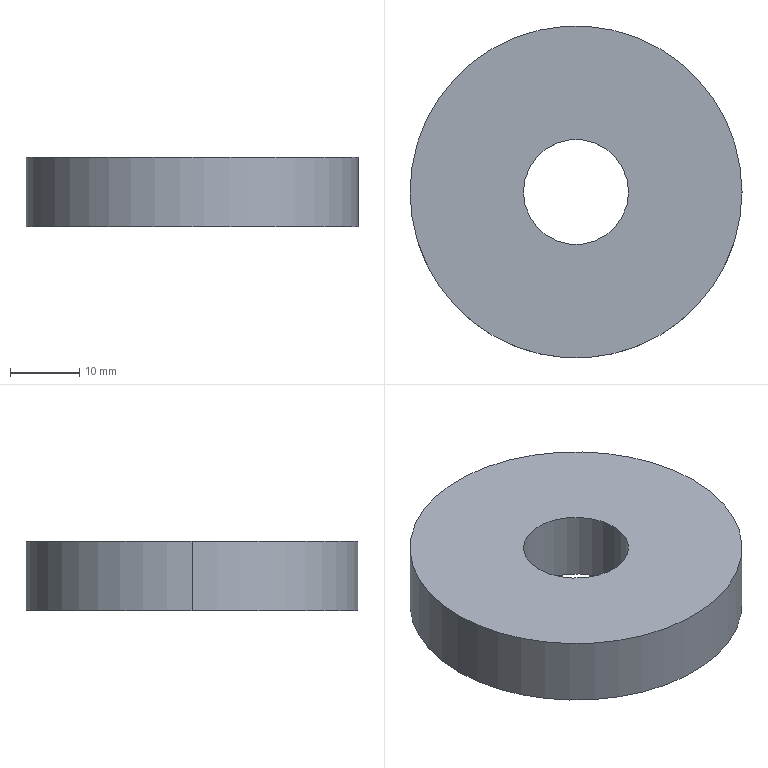Part | SolidWorks | features Extrusion 1 | 1 solid | 6 faces | box 48 x 48 x 10 mm | volume 16281 mm3 | cylinder 4 | plane 2 | commonest cylinder face diameters 15.2 x2 48 x2
STEP:
#1=CARTESIAN_POINT('',(-7.6,0.,10.));
#2=VERTEX_POINT('',#1);
#3=CARTESIAN_POINT('',(7.6,0.,10.));
#4=VERTEX_POINT('',#3);
#5=CARTESIAN_POINT('',(0.,0.,10.));
#6=DIRECTION('',(0.,0.,1.));
#7=DIRECTION('',(1.,0.,0.));
#8=AXIS2_PLACEMENT_3D('',#5,#6,#7);
#9=CIRCLE('',#8,7.6);
#10=EDGE_CURVE('',#2,#4,#9,.T.);
#11=ORIENTED_EDGE('',*,*,#10,.T.);
#12=CARTESIAN_POINT('',(7.6,0.,0.));
#13=VERTEX_POINT('',#12);
#14=CARTESIAN_POINT('',(7.6,0.,10.));
#15=DIRECTION('',(0.,0.,-1.));
#16=VECTOR('',#15,1000.);
#17=LINE('',#14,#16);
#18=EDGE_CURVE('',#4,#13,#17,.T.);
#19=ORIENTED_EDGE('',*,*,#18,.T.);
#20=CARTESIAN_POINT('',(-7.6,0.,0.));
#21=VERTEX_POINT('',#20);
#22=CARTESIAN_POINT('',(0.,0.,0.));
#23=DIRECTION('',(0.,0.,1.));
#24=DIRECTION('',(1.,0.,0.));
#25=AXIS2_PLACEMENT_3D('',#22,#23,#24);
#26=CIRCLE('',#25,7.6);
#27=EDGE_CURVE('',#21,#13,#26,.T.);
#28=ORIENTED_EDGE('',*,*,#27,.F.);
#29=CARTESIAN_POINT('',(-7.6,0.,10.));
#30=DIRECTION('',(0.,0.,-1.));
#31=VECTOR('',#30,1000.);
#32=LINE('',#29,#31);
#33=EDGE_CURVE('',#2,#21,#32,.T.);
#34=ORIENTED_EDGE('',*,*,#33,.F.);
#35=EDGE_LOOP('',(#11,#19,#28,#34));
#36=FACE_OUTER_BOUND('',#35,.T.);
#37=CARTESIAN_POINT('',(0.,0.,10.));
#38=DIRECTION('',(0.,0.,-1.));
#39=DIRECTION('',(-1.,0.,0.));
#40=AXIS2_PLACEMENT_3D('',#37,#38,#39);
#41=CYLINDRICAL_SURFACE('',#40,7.6);
#42=ADVANCED_FACE('',(#36),#41,.F.);
#43=CARTESIAN_POINT('',(24.,0.,10.));
#44=VERTEX_POINT('',#43);
#45=CARTESIAN_POINT('',(-24.,0.,10.));
#46=VERTEX_POINT('',#45);
#47=CARTESIAN_POINT('',(0.,0.,10.));
#48=DIRECTION('',(0.,0.,1.));
#49=DIRECTION('',(1.,0.,0.));
#50=AXIS2_PLACEMENT_3D('',#47,#48,#49);
#51=CIRCLE('',#50,24.);
#52=EDGE_CURVE('',#44,#46,#51,.T.);
#53=ORIENTED_EDGE('',*,*,#52,.F.);
#54=CARTESIAN_POINT('',(24.,0.,0.));
#55=VERTEX_POINT('',#54);
#56=CARTESIAN_POINT('',(24.,0.,10.));
#57=DIRECTION('',(0.,0.,-1.));
#58=VECTOR('',#57,1000.);
#59=LINE('',#56,#58);
#60=EDGE_CURVE('',#44,#55,#59,.T.);
#61=ORIENTED_EDGE('',*,*,#60,.T.);
#62=CARTESIAN_POINT('',(-24.,0.,0.));
#63=VERTEX_POINT('',#62);
#64=CARTESIAN_POINT('',(0.,0.,0.));
#65=DIRECTION('',(0.,0.,1.));
#66=DIRECTION('',(1.,0.,0.));
#67=AXIS2_PLACEMENT_3D('',#64,#65,#66);
#68=CIRCLE('',#67,24.);
#69=EDGE_CURVE('',#55,#63,#68,.T.);
#70=ORIENTED_EDGE('',*,*,#69,.T.);
#71=CARTESIAN_POINT('',(-24.,0.,10.));
#72=DIRECTION('',(0.,0.,-1.));
#73=VECTOR('',#72,1000.);
#74=LINE('',#71,#73);
#75=EDGE_CURVE('',#46,#63,#74,.T.);
#76=ORIENTED_EDGE('',*,*,#75,.F.);
#77=EDGE_LOOP('',(#53,#61,#70,#76));
#78=FACE_OUTER_BOUND('',#77,.T.);
#79=CARTESIAN_POINT('',(0.,0.,10.));
#80=DIRECTION('',(0.,0.,-1.));
#81=DIRECTION('',(-1.,0.,0.));
#82=AXIS2_PLACEMENT_3D('',#79,#80,#81);
#83=CYLINDRICAL_SURFACE('',#82,24.);
#84=ADVANCED_FACE('',(#78),#83,.T.);
#85=CARTESIAN_POINT('',(0.,0.,10.));
#86=DIRECTION('',(0.,0.,1.));
#87=DIRECTION('',(1.,0.,0.));
#88=AXIS2_PLACEMENT_3D('',#85,#86,#87);
#89=CIRCLE('',#88,24.);
#90=EDGE_CURVE('',#46,#44,#89,.T.);
#91=ORIENTED_EDGE('',*,*,#90,.T.);
#92=ORIENTED_EDGE('',*,*,#52,.T.);
#93=EDGE_LOOP('',(#91,#92));
#94=FACE_OUTER_BOUND('',#93,.T.);
#95=ORIENTED_EDGE('',*,*,#10,.F.);
#96=CARTESIAN_POINT('',(0.,0.,10.));
#97=DIRECTION('',(0.,0.,1.));
#98=DIRECTION('',(1.,0.,0.));
#99=AXIS2_PLACEMENT_3D('',#96,#97,#98);
#100=CIRCLE('',#99,7.6);
#101=EDGE_CURVE('',#4,#2,#100,.T.);
#102=ORIENTED_EDGE('',*,*,#101,.F.);
#103=EDGE_LOOP('',(#95,#102));
#104=FACE_BOUND('',#103,.T.);
#105=CARTESIAN_POINT('',(0.,0.,10.));
#106=DIRECTION('',(0.,0.,1.));
#107=DIRECTION('',(1.,0.,0.));
#108=AXIS2_PLACEMENT_3D('',#105,#106,#107);
#109=PLANE('',#108);
#110=ADVANCED_FACE('',(#94,#104),#109,.T.);
#111=CARTESIAN_POINT('',(0.,0.,0.));
#112=DIRECTION('',(0.,0.,1.));
#113=DIRECTION('',(1.,0.,0.));
#114=AXIS2_PLACEMENT_3D('',#111,#112,#113);
#115=CIRCLE('',#114,24.);
#116=EDGE_CURVE('',#63,#55,#115,.T.);
#117=ORIENTED_EDGE('',*,*,#116,.F.);
#118=ORIENTED_EDGE('',*,*,#69,.F.);
#119=EDGE_LOOP('',(#117,#118));
#120=FACE_OUTER_BOUND('',#119,.T.);
#121=ORIENTED_EDGE('',*,*,#27,.T.);
#122=CARTESIAN_POINT('',(0.,0.,0.));
#123=DIRECTION('',(0.,0.,1.));
#124=DIRECTION('',(1.,0.,0.));
#125=AXIS2_PLACEMENT_3D('',#122,#123,#124);
#126=CIRCLE('',#125,7.6);
#127=EDGE_CURVE('',#13,#21,#126,.T.);
#128=ORIENTED_EDGE('',*,*,#127,.T.);
#129=EDGE_LOOP('',(#121,#128));
#130=FACE_BOUND('',#129,.T.);
#131=CARTESIAN_POINT('',(0.,0.,0.));
#132=DIRECTION('',(0.,0.,1.));
#133=DIRECTION('',(1.,0.,0.));
#134=AXIS2_PLACEMENT_3D('',#131,#132,#133);
#135=PLANE('',#134);
#136=ADVANCED_FACE('',(#120,#130),#135,.F.);
#137=ORIENTED_EDGE('',*,*,#60,.F.);
#138=ORIENTED_EDGE('',*,*,#90,.F.);
#139=ORIENTED_EDGE('',*,*,#75,.T.);
#140=ORIENTED_EDGE('',*,*,#116,.T.);
#141=EDGE_LOOP('',(#137,#138,#139,#140));
#142=FACE_OUTER_BOUND('',#141,.T.);
#143=CARTESIAN_POINT('',(0.,0.,10.));
#144=DIRECTION('',(0.,0.,-1.));
#145=DIRECTION('',(-1.,0.,0.));
#146=AXIS2_PLACEMENT_3D('',#143,#144,#145);
#147=CYLINDRICAL_SURFACE('',#146,24.);
#148=ADVANCED_FACE('',(#142),#147,.T.);
#149=ORIENTED_EDGE('',*,*,#18,.F.);
#150=ORIENTED_EDGE('',*,*,#101,.T.);
#151=ORIENTED_EDGE('',*,*,#33,.T.);
#152=ORIENTED_EDGE('',*,*,#127,.F.);
#153=EDGE_LOOP('',(#149,#150,#151,#152));
#154=FACE_OUTER_BOUND('',#153,.T.);
#155=CARTESIAN_POINT('',(0.,0.,10.));
#156=DIRECTION('',(0.,0.,-1.));
#157=DIRECTION('',(-1.,0.,0.));
#158=AXIS2_PLACEMENT_3D('',#155,#156,#157);
#159=CYLINDRICAL_SURFACE('',#158,7.6);
#160=ADVANCED_FACE('',(#154),#159,.F.);
#161=CLOSED_SHELL('',(#42,#84,#110,#136,#148,#160));
#162=MANIFOLD_SOLID_BREP('',#161);
#163=CARTESIAN_POINT('',(0.,0.,0.));
#164=DIRECTION('',(0.,0.,1.));
#165=DIRECTION('',(1.,0.,0.));
#166=AXIS2_PLACEMENT_3D('',#163,#164,#165);
#167=(LENGTH_UNIT()NAMED_UNIT(*)SI_UNIT(.MILLI.,.METRE.));
#168=UNCERTAINTY_MEASURE_WITH_UNIT(LENGTH_MEASURE(0.00001),#167,'','');
#169=(NAMED_UNIT(*)PLANE_ANGLE_UNIT()SI_UNIT($,.RADIAN.));
#170=(NAMED_UNIT(*)SI_UNIT($,.STERADIAN.)SOLID_ANGLE_UNIT());
#171=(GEOMETRIC_REPRESENTATION_CONTEXT(3)GLOBAL_UNCERTAINTY_ASSIGNED_CONTEXT((#168))GLOBAL_UNIT_ASSIGNED_CONTEXT((#167,#169,#170))REPRESENTATION_CONTEXT('',''));
#172=ADVANCED_BREP_SHAPE_REPRESENTATION('',(#162,#166),#171);